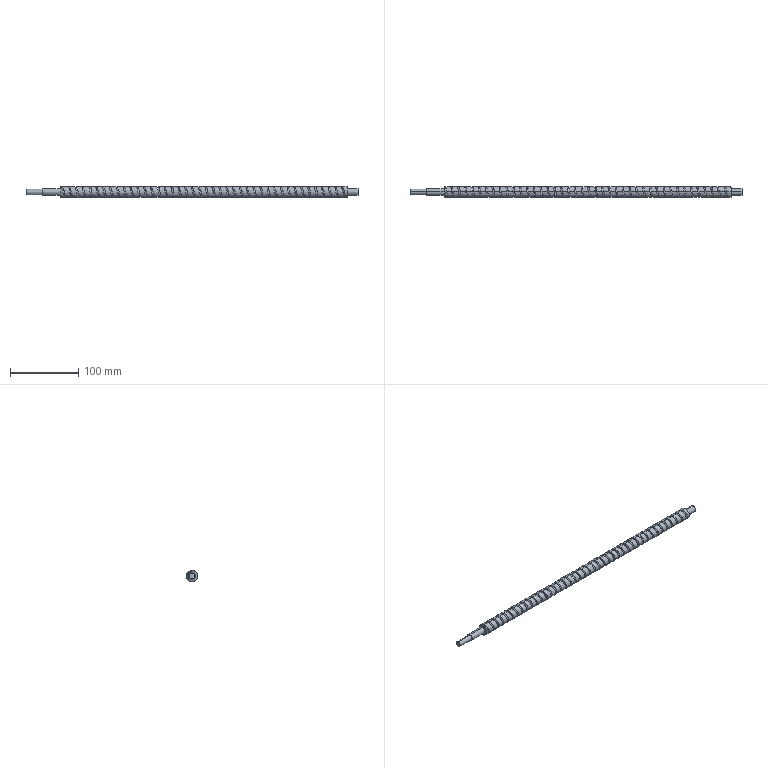Part | SolidWorks | features BaseBody 1 | 1 solid | 117 faces | box 486 x 16 x 16 mm | volume 83136 mm3 | cylinder 93 | spline 19 | plane 5 | commonest cylinder face diameters 16 x87 10 x4 8 x2